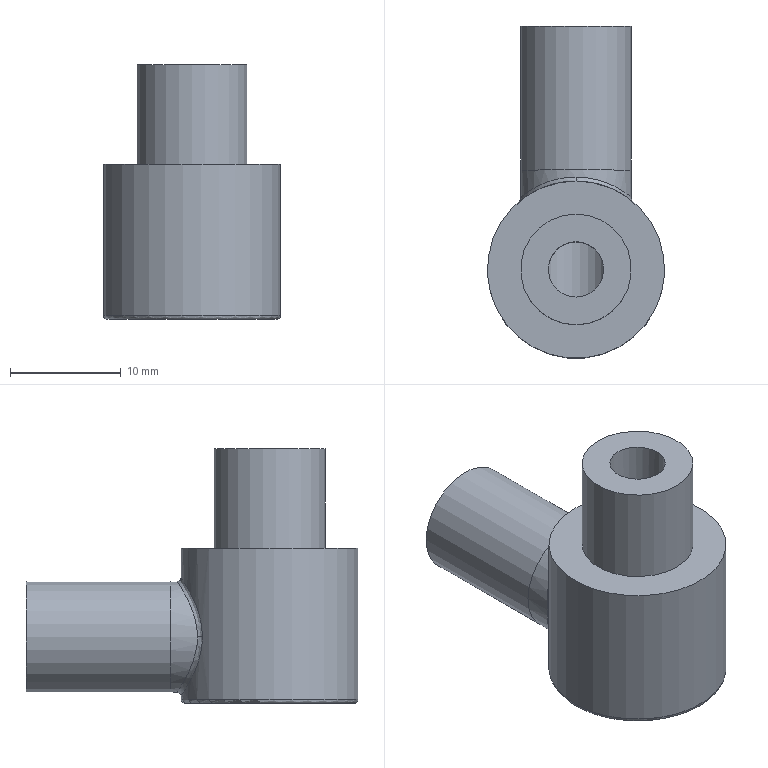Part | STEP file | 1-55.3 | 1 solid | 15 faces | box 16 x 30 x 23 mm | volume 3666 mm3 | cylinder 6 | plane 5 | spline 3 | torus 1 | commonest cylinder face diameters 10 x3 5 x1 6 x1 16 x1